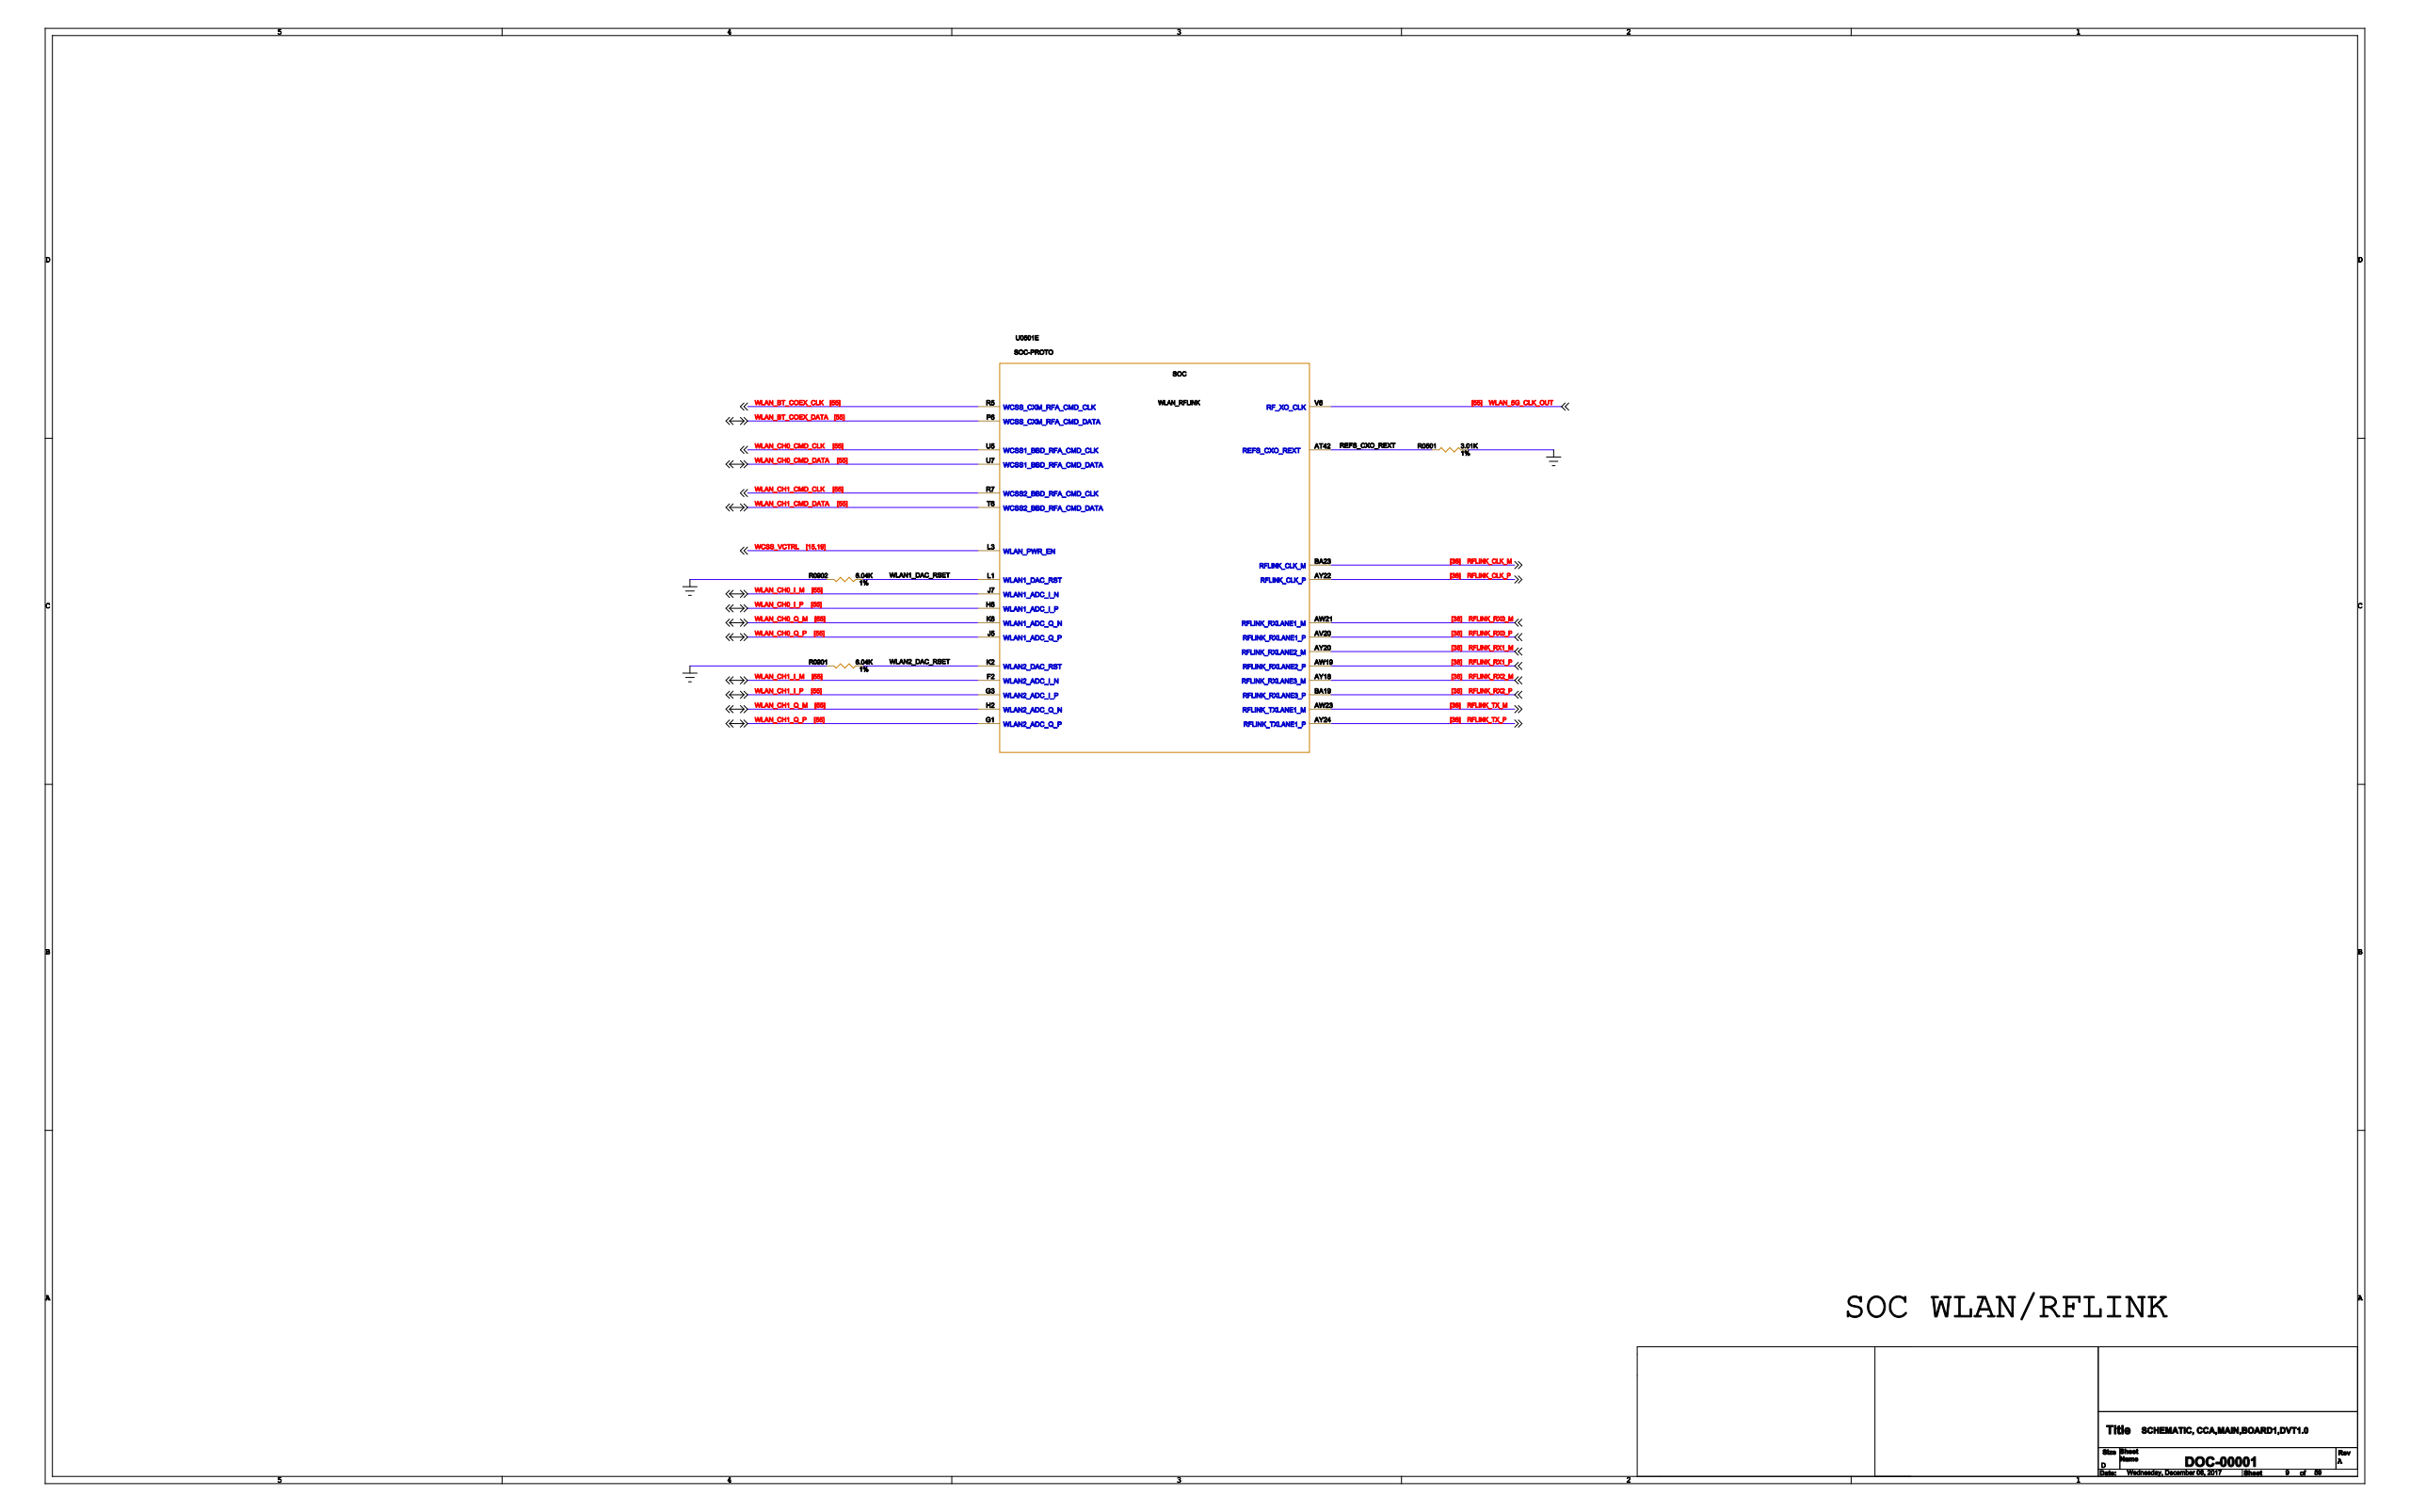Circuit board | KiCad | 1657 parts | 1365 nets | one sheet of the schematic
Parts on this sheet (reference | value | footprint):
R0501
R0901
R0902
U0501
Nets of these parts (net: part-pin ...):
GND: R0501-1 R0901-1 R0902-1
REFS_CXO_REXT: R0501-2 U0501-AT42
WLAN1_DAC_RSET: R0901-2 U0501-K2
WLAN_CH0_Q_M: U0501-K6
WLAN_CH0_I_M: U0501-J7
WLAN_CH0_I_P: U0501-H6
WLAN_CH0_Q_P: U0501-J5
WLAN_CH1_Q_M: U0501-H2
WLAN_CH1_I_M: U0501-F2
WLAN_CH1_Q_P: U0501-G1
WLAN_CH1_I_P: U0501-G3
WLAN2_DAC_RSET: R0902-2 U0501-L1
RFLINK_RX0_P: U0501-AV20
RFLINK_RX1_P: U0501-AW19
RFLINK_RX0_M: U0501-AW21
RFLINK_TX_M: U0501-AW23
RFLINK_RX2_M: U0501-AY18
RFLINK_RX1_M: U0501-AY20
RFLINK_CLK_P: U0501-AY22
RFLINK_TX_P: U0501-AY24
RFLINK_RX2_P: U0501-BA19
RFLINK_CLK_M: U0501-BA23
WCSS_VCTRL: U0501-L3